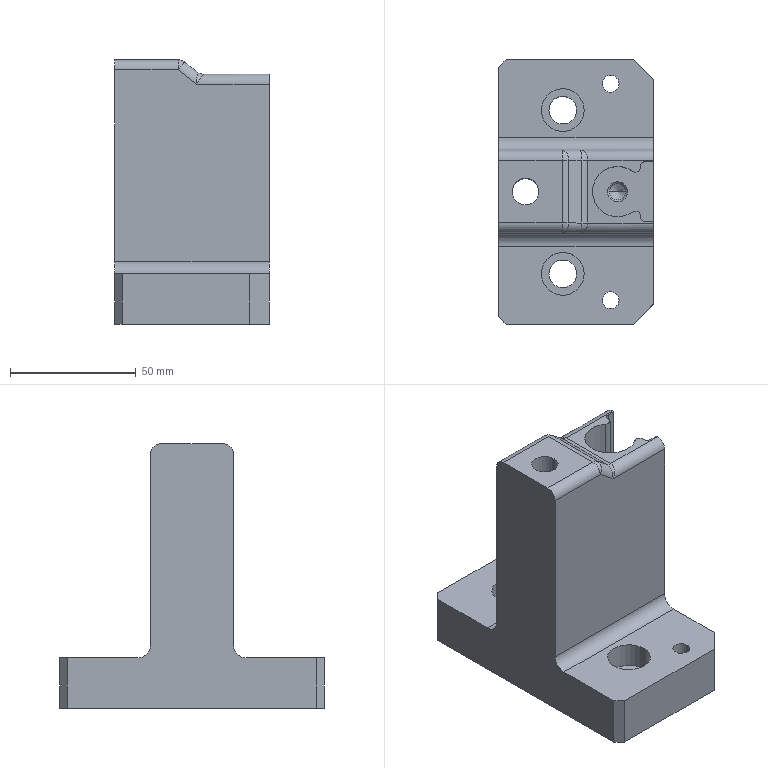Part | STEP file | 1_id1590_x_t | 1 solid | 62 faces | box 61.499 x 105 x 105 mm | volume 262460 mm3 | cylinder 31 | plane 23 | cone 4 | sphere 2 | spline 2 | commonest cylinder face diameters 8 x8 4 x4 6.75 x4 11 x4 17 x4 6.528 x2